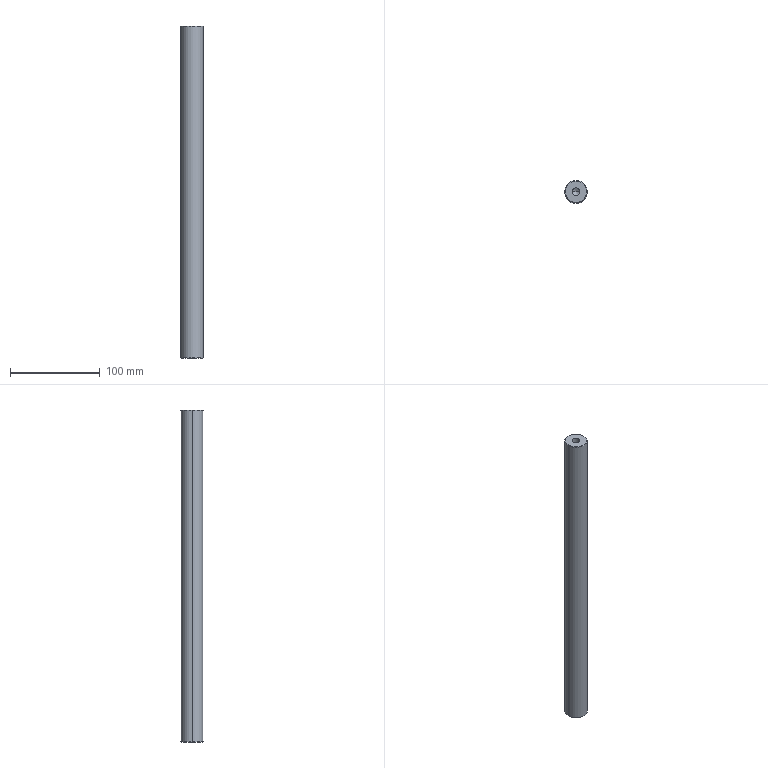Part | STEP file | 03-27 post B | 1 solid | 16 faces | box 25 x 25 x 370 mm | volume 178727 mm3 | cone 8 | cylinder 6 | plane 2 | commonest cylinder face diameters 8.5 x4 25 x2
STEP:
#1=CARTESIAN_POINT('',(4.25,0.,24.5));
#2=VERTEX_POINT('',#1);
#3=CARTESIAN_POINT('',(-4.25,0.,24.5));
#4=VERTEX_POINT('',#3);
#5=CARTESIAN_POINT('',(0.,0.,24.5));
#6=DIRECTION('',(0.,0.,-1.));
#7=DIRECTION('',(-1.,0.,0.));
#8=AXIS2_PLACEMENT_3D('',#5,#6,#7);
#9=CIRCLE('',#8,4.25);
#10=EDGE_CURVE('',#2,#4,#9,.T.);
#11=ORIENTED_EDGE('',*,*,#10,.F.);
#12=CARTESIAN_POINT('',(4.25,0.,0.));
#13=VERTEX_POINT('',#12);
#14=CARTESIAN_POINT('',(4.25,0.,0.));
#15=DIRECTION('',(0.,0.,-1.));
#16=VECTOR('',#15,1000.);
#17=LINE('',#14,#16);
#18=EDGE_CURVE('',#2,#13,#17,.T.);
#19=ORIENTED_EDGE('',*,*,#18,.T.);
#20=CARTESIAN_POINT('',(-4.25,0.,0.));
#21=VERTEX_POINT('',#20);
#22=CARTESIAN_POINT('',(0.,0.,0.));
#23=DIRECTION('',(0.,0.,-1.));
#24=DIRECTION('',(-1.,0.,0.));
#25=AXIS2_PLACEMENT_3D('',#22,#23,#24);
#26=CIRCLE('',#25,4.25);
#27=EDGE_CURVE('',#13,#21,#26,.T.);
#28=ORIENTED_EDGE('',*,*,#27,.T.);
#29=CARTESIAN_POINT('',(-4.25,0.,0.));
#30=DIRECTION('',(0.,0.,-1.));
#31=VECTOR('',#30,1000.);
#32=LINE('',#29,#31);
#33=EDGE_CURVE('',#4,#21,#32,.T.);
#34=ORIENTED_EDGE('',*,*,#33,.F.);
#35=EDGE_LOOP('',(#11,#19,#28,#34));
#36=FACE_OUTER_BOUND('',#35,.T.);
#37=CARTESIAN_POINT('',(0.,0.,0.));
#38=DIRECTION('',(0.,0.,-1.));
#39=DIRECTION('',(-1.,0.,0.));
#40=AXIS2_PLACEMENT_3D('',#37,#38,#39);
#41=CYLINDRICAL_SURFACE('',#40,4.25);
#42=ADVANCED_FACE('',(#36),#41,.F.);
#43=CARTESIAN_POINT('',(0.,0.,27.054));
#44=VERTEX_POINT('',#43);
#45=CARTESIAN_POINT('',(-4.25,0.,24.5));
#46=DIRECTION('',(-0.8572,0.,-0.515));
#47=VECTOR('',#46,1000.);
#48=LINE('',#45,#47);
#49=EDGE_CURVE('',#44,#4,#48,.T.);
#50=ORIENTED_EDGE('',*,*,#49,.F.);
#51=CARTESIAN_POINT('',(4.25,0.,24.5));
#52=DIRECTION('',(0.8572,0.,-0.515));
#53=VECTOR('',#52,1000.);
#54=LINE('',#51,#53);
#55=EDGE_CURVE('',#44,#2,#54,.T.);
#56=ORIENTED_EDGE('',*,*,#55,.T.);
#57=ORIENTED_EDGE('',*,*,#10,.T.);
#58=EDGE_LOOP('',(#50,#56,#57));
#59=FACE_OUTER_BOUND('',#58,.T.);
#60=CARTESIAN_POINT('',(0.,0.,24.5));
#61=DIRECTION('',(0.,0.,-1.));
#62=DIRECTION('',(-1.,0.,0.));
#63=AXIS2_PLACEMENT_3D('',#60,#61,#62);
#64=CONICAL_SURFACE('',#63,4.25,1.03);
#65=ADVANCED_FACE('',(#59),#64,.F.);
#66=CARTESIAN_POINT('',(-4.25,0.,345.5));
#67=VERTEX_POINT('',#66);
#68=CARTESIAN_POINT('',(4.25,0.,345.5));
#69=VERTEX_POINT('',#68);
#70=CARTESIAN_POINT('',(0.,0.,345.5));
#71=DIRECTION('',(0.,0.,1.));
#72=DIRECTION('',(1.,0.,0.));
#73=AXIS2_PLACEMENT_3D('',#70,#71,#72);
#74=CIRCLE('',#73,4.25);
#75=EDGE_CURVE('',#67,#69,#74,.T.);
#76=ORIENTED_EDGE('',*,*,#75,.F.);
#77=CARTESIAN_POINT('',(-4.25,0.,370.));
#78=VERTEX_POINT('',#77);
#79=CARTESIAN_POINT('',(-4.25,0.,370.));
#80=DIRECTION('',(0.,0.,1.));
#81=VECTOR('',#80,1000.);
#82=LINE('',#79,#81);
#83=EDGE_CURVE('',#67,#78,#82,.T.);
#84=ORIENTED_EDGE('',*,*,#83,.T.);
#85=CARTESIAN_POINT('',(4.25,0.,370.));
#86=VERTEX_POINT('',#85);
#87=CARTESIAN_POINT('',(0.,0.,370.));
#88=DIRECTION('',(0.,0.,1.));
#89=DIRECTION('',(1.,0.,0.));
#90=AXIS2_PLACEMENT_3D('',#87,#88,#89);
#91=CIRCLE('',#90,4.25);
#92=EDGE_CURVE('',#78,#86,#91,.T.);
#93=ORIENTED_EDGE('',*,*,#92,.T.);
#94=CARTESIAN_POINT('',(4.25,0.,370.));
#95=DIRECTION('',(0.,0.,1.));
#96=VECTOR('',#95,1000.);
#97=LINE('',#94,#96);
#98=EDGE_CURVE('',#69,#86,#97,.T.);
#99=ORIENTED_EDGE('',*,*,#98,.F.);
#100=EDGE_LOOP('',(#76,#84,#93,#99));
#101=FACE_OUTER_BOUND('',#100,.T.);
#102=CARTESIAN_POINT('',(0.,0.,370.));
#103=DIRECTION('',(0.,0.,1.));
#104=DIRECTION('',(1.,0.,0.));
#105=AXIS2_PLACEMENT_3D('',#102,#103,#104);
#106=CYLINDRICAL_SURFACE('',#105,4.25);
#107=ADVANCED_FACE('',(#101),#106,.F.);
#108=CARTESIAN_POINT('',(0.,0.,342.946));
#109=VERTEX_POINT('',#108);
#110=CARTESIAN_POINT('',(4.25,0.,345.5));
#111=DIRECTION('',(0.8572,0.,0.515));
#112=VECTOR('',#111,1000.);
#113=LINE('',#110,#112);
#114=EDGE_CURVE('',#109,#69,#113,.T.);
#115=ORIENTED_EDGE('',*,*,#114,.F.);
#116=CARTESIAN_POINT('',(-4.25,0.,345.5));
#117=DIRECTION('',(-0.8572,0.,0.515));
#118=VECTOR('',#117,1000.);
#119=LINE('',#116,#118);
#120=EDGE_CURVE('',#109,#67,#119,.T.);
#121=ORIENTED_EDGE('',*,*,#120,.T.);
#122=ORIENTED_EDGE('',*,*,#75,.T.);
#123=EDGE_LOOP('',(#115,#121,#122));
#124=FACE_OUTER_BOUND('',#123,.T.);
#125=CARTESIAN_POINT('',(0.,0.,345.5));
#126=DIRECTION('',(0.,0.,1.));
#127=DIRECTION('',(1.,0.,0.));
#128=AXIS2_PLACEMENT_3D('',#125,#126,#127);
#129=CONICAL_SURFACE('',#128,4.25,1.03);
#130=ADVANCED_FACE('',(#124),#129,.F.);
#131=CARTESIAN_POINT('',(12.,0.,370.));
#132=VERTEX_POINT('',#131);
#133=CARTESIAN_POINT('',(-12.,0.,370.));
#134=VERTEX_POINT('',#133);
#135=CARTESIAN_POINT('',(0.,0.,370.));
#136=DIRECTION('',(0.,0.,1.));
#137=DIRECTION('',(1.,0.,0.));
#138=AXIS2_PLACEMENT_3D('',#135,#136,#137);
#139=CIRCLE('',#138,12.);
#140=EDGE_CURVE('',#132,#134,#139,.T.);
#141=ORIENTED_EDGE('',*,*,#140,.F.);
#142=CARTESIAN_POINT('',(12.5,0.,369.5));
#143=VERTEX_POINT('',#142);
#144=CARTESIAN_POINT('',(12.,0.,370.));
#145=DIRECTION('',(0.7071,0.,-0.7071));
#146=VECTOR('',#145,1000.);
#147=LINE('',#144,#146);
#148=EDGE_CURVE('',#132,#143,#147,.T.);
#149=ORIENTED_EDGE('',*,*,#148,.T.);
#150=CARTESIAN_POINT('',(-12.5,0.,369.5));
#151=VERTEX_POINT('',#150);
#152=CARTESIAN_POINT('',(0.,0.,369.5));
#153=DIRECTION('',(0.,0.,-1.));
#154=DIRECTION('',(1.,0.,0.));
#155=AXIS2_PLACEMENT_3D('',#152,#153,#154);
#156=CIRCLE('',#155,12.5);
#157=EDGE_CURVE('',#151,#143,#156,.T.);
#158=ORIENTED_EDGE('',*,*,#157,.F.);
#159=CARTESIAN_POINT('',(-12.,0.,370.));
#160=DIRECTION('',(-0.7071,0.,-0.7071));
#161=VECTOR('',#160,1000.);
#162=LINE('',#159,#161);
#163=EDGE_CURVE('',#134,#151,#162,.T.);
#164=ORIENTED_EDGE('',*,*,#163,.F.);
#165=EDGE_LOOP('',(#141,#149,#158,#164));
#166=FACE_OUTER_BOUND('',#165,.T.);
#167=CARTESIAN_POINT('',(0.,0.,370.));
#168=DIRECTION('',(0.,0.,-1.));
#169=DIRECTION('',(-1.,0.,0.));
#170=AXIS2_PLACEMENT_3D('',#167,#168,#169);
#171=CONICAL_SURFACE('',#170,12.,0.7854);
#172=ADVANCED_FACE('',(#166),#171,.T.);
#173=CARTESIAN_POINT('',(-12.,0.,0.));
#174=VERTEX_POINT('',#173);
#175=CARTESIAN_POINT('',(12.,0.,0.));
#176=VERTEX_POINT('',#175);
#177=CARTESIAN_POINT('',(0.,0.,0.));
#178=DIRECTION('',(0.,0.,-1.));
#179=DIRECTION('',(1.,0.,0.));
#180=AXIS2_PLACEMENT_3D('',#177,#178,#179);
#181=CIRCLE('',#180,12.);
#182=EDGE_CURVE('',#174,#176,#181,.T.);
#183=ORIENTED_EDGE('',*,*,#182,.F.);
#184=CARTESIAN_POINT('',(-12.5,0.,0.5));
#185=VERTEX_POINT('',#184);
#186=CARTESIAN_POINT('',(-12.5,0.,0.5));
#187=DIRECTION('',(-0.7071,0.,0.7071));
#188=VECTOR('',#187,1000.);
#189=LINE('',#186,#188);
#190=EDGE_CURVE('',#174,#185,#189,.T.);
#191=ORIENTED_EDGE('',*,*,#190,.T.);
#192=CARTESIAN_POINT('',(12.5,0.,0.5));
#193=VERTEX_POINT('',#192);
#194=CARTESIAN_POINT('',(0.,0.,0.5));
#195=DIRECTION('',(0.,0.,1.));
#196=DIRECTION('',(1.,0.,0.));
#197=AXIS2_PLACEMENT_3D('',#194,#195,#196);
#198=CIRCLE('',#197,12.5);
#199=EDGE_CURVE('',#193,#185,#198,.T.);
#200=ORIENTED_EDGE('',*,*,#199,.F.);
#201=CARTESIAN_POINT('',(12.5,0.,0.5));
#202=DIRECTION('',(0.7071,0.,0.7071));
#203=VECTOR('',#202,1000.);
#204=LINE('',#201,#203);
#205=EDGE_CURVE('',#176,#193,#204,.T.);
#206=ORIENTED_EDGE('',*,*,#205,.F.);
#207=EDGE_LOOP('',(#183,#191,#200,#206));
#208=FACE_OUTER_BOUND('',#207,.T.);
#209=CARTESIAN_POINT('',(0.,0.,0.5));
#210=DIRECTION('',(0.,0.,1.));
#211=DIRECTION('',(1.,0.,0.));
#212=AXIS2_PLACEMENT_3D('',#209,#210,#211);
#213=CONICAL_SURFACE('',#212,12.5,0.7854);
#214=ADVANCED_FACE('',(#208),#213,.T.);
#215=ORIENTED_EDGE('',*,*,#157,.T.);
#216=CARTESIAN_POINT('',(12.5,0.,370.));
#217=DIRECTION('',(0.,0.,-1.));
#218=VECTOR('',#217,1000.);
#219=LINE('',#216,#218);
#220=EDGE_CURVE('',#143,#193,#219,.T.);
#221=ORIENTED_EDGE('',*,*,#220,.T.);
#222=ORIENTED_EDGE('',*,*,#199,.T.);
#223=CARTESIAN_POINT('',(-12.5,0.,370.));
#224=DIRECTION('',(0.,0.,-1.));
#225=VECTOR('',#224,1000.);
#226=LINE('',#223,#225);
#227=EDGE_CURVE('',#151,#185,#226,.T.);
#228=ORIENTED_EDGE('',*,*,#227,.F.);
#229=EDGE_LOOP('',(#215,#221,#222,#228));
#230=FACE_OUTER_BOUND('',#229,.T.);
#231=CARTESIAN_POINT('',(0.,0.,370.));
#232=DIRECTION('',(0.,0.,-1.));
#233=DIRECTION('',(-1.,0.,0.));
#234=AXIS2_PLACEMENT_3D('',#231,#232,#233);
#235=CYLINDRICAL_SURFACE('',#234,12.5);
#236=ADVANCED_FACE('',(#230),#235,.T.);
#237=ORIENTED_EDGE('',*,*,#220,.F.);
#238=CARTESIAN_POINT('',(0.,0.,369.5));
#239=DIRECTION('',(0.,0.,-1.));
#240=DIRECTION('',(1.,0.,0.));
#241=AXIS2_PLACEMENT_3D('',#238,#239,#240);
#242=CIRCLE('',#241,12.5);
#243=EDGE_CURVE('',#143,#151,#242,.T.);
#244=ORIENTED_EDGE('',*,*,#243,.T.);
#245=ORIENTED_EDGE('',*,*,#227,.T.);
#246=CARTESIAN_POINT('',(0.,0.,0.5));
#247=DIRECTION('',(0.,0.,1.));
#248=DIRECTION('',(1.,0.,0.));
#249=AXIS2_PLACEMENT_3D('',#246,#247,#248);
#250=CIRCLE('',#249,12.5);
#251=EDGE_CURVE('',#185,#193,#250,.T.);
#252=ORIENTED_EDGE('',*,*,#251,.T.);
#253=EDGE_LOOP('',(#237,#244,#245,#252));
#254=FACE_OUTER_BOUND('',#253,.T.);
#255=CARTESIAN_POINT('',(0.,0.,370.));
#256=DIRECTION('',(0.,0.,-1.));
#257=DIRECTION('',(-1.,0.,0.));
#258=AXIS2_PLACEMENT_3D('',#255,#256,#257);
#259=CYLINDRICAL_SURFACE('',#258,12.5);
#260=ADVANCED_FACE('',(#254),#259,.T.);
#261=CARTESIAN_POINT('',(0.,0.,370.));
#262=DIRECTION('',(0.,0.,1.));
#263=DIRECTION('',(1.,0.,0.));
#264=AXIS2_PLACEMENT_3D('',#261,#262,#263);
#265=CIRCLE('',#264,4.25);
#266=EDGE_CURVE('',#86,#78,#265,.T.);
#267=ORIENTED_EDGE('',*,*,#266,.F.);
#268=ORIENTED_EDGE('',*,*,#92,.F.);
#269=EDGE_LOOP('',(#267,#268));
#270=FACE_BOUND('',#269,.T.);
#271=CARTESIAN_POINT('',(0.,0.,370.));
#272=DIRECTION('',(0.,0.,1.));
#273=DIRECTION('',(1.,0.,0.));
#274=AXIS2_PLACEMENT_3D('',#271,#272,#273);
#275=CIRCLE('',#274,12.);
#276=EDGE_CURVE('',#134,#132,#275,.T.);
#277=ORIENTED_EDGE('',*,*,#276,.T.);
#278=ORIENTED_EDGE('',*,*,#140,.T.);
#279=EDGE_LOOP('',(#277,#278));
#280=FACE_OUTER_BOUND('',#279,.T.);
#281=CARTESIAN_POINT('',(0.,0.,370.));
#282=DIRECTION('',(0.,0.,1.));
#283=DIRECTION('',(1.,0.,0.));
#284=AXIS2_PLACEMENT_3D('',#281,#282,#283);
#285=PLANE('',#284);
#286=ADVANCED_FACE('',(#270,#280),#285,.T.);
#287=CARTESIAN_POINT('',(0.,0.,0.));
#288=DIRECTION('',(0.,0.,-1.));
#289=DIRECTION('',(-1.,0.,0.));
#290=AXIS2_PLACEMENT_3D('',#287,#288,#289);
#291=CIRCLE('',#290,4.25);
#292=EDGE_CURVE('',#21,#13,#291,.T.);
#293=ORIENTED_EDGE('',*,*,#292,.F.);
#294=ORIENTED_EDGE('',*,*,#27,.F.);
#295=EDGE_LOOP('',(#293,#294));
#296=FACE_BOUND('',#295,.T.);
#297=CARTESIAN_POINT('',(0.,0.,0.));
#298=DIRECTION('',(0.,0.,-1.));
#299=DIRECTION('',(1.,0.,0.));
#300=AXIS2_PLACEMENT_3D('',#297,#298,#299);
#301=CIRCLE('',#300,12.);
#302=EDGE_CURVE('',#176,#174,#301,.T.);
#303=ORIENTED_EDGE('',*,*,#302,.T.);
#304=ORIENTED_EDGE('',*,*,#182,.T.);
#305=EDGE_LOOP('',(#303,#304));
#306=FACE_OUTER_BOUND('',#305,.T.);
#307=CARTESIAN_POINT('',(0.,0.,0.));
#308=DIRECTION('',(0.,0.,1.));
#309=DIRECTION('',(1.,0.,0.));
#310=AXIS2_PLACEMENT_3D('',#307,#308,#309);
#311=PLANE('',#310);
#312=ADVANCED_FACE('',(#296,#306),#311,.F.);
#313=ORIENTED_EDGE('',*,*,#190,.F.);
#314=ORIENTED_EDGE('',*,*,#302,.F.);
#315=ORIENTED_EDGE('',*,*,#205,.T.);
#316=ORIENTED_EDGE('',*,*,#251,.F.);
#317=EDGE_LOOP('',(#313,#314,#315,#316));
#318=FACE_OUTER_BOUND('',#317,.T.);
#319=CARTESIAN_POINT('',(0.,0.,0.5));
#320=DIRECTION('',(0.,0.,1.));
#321=DIRECTION('',(1.,0.,0.));
#322=AXIS2_PLACEMENT_3D('',#319,#320,#321);
#323=CONICAL_SURFACE('',#322,12.5,0.7854);
#324=ADVANCED_FACE('',(#318),#323,.T.);
#325=ORIENTED_EDGE('',*,*,#148,.F.);
#326=ORIENTED_EDGE('',*,*,#276,.F.);
#327=ORIENTED_EDGE('',*,*,#163,.T.);
#328=ORIENTED_EDGE('',*,*,#243,.F.);
#329=EDGE_LOOP('',(#325,#326,#327,#328));
#330=FACE_OUTER_BOUND('',#329,.T.);
#331=CARTESIAN_POINT('',(0.,0.,370.));
#332=DIRECTION('',(0.,0.,-1.));
#333=DIRECTION('',(-1.,0.,0.));
#334=AXIS2_PLACEMENT_3D('',#331,#332,#333);
#335=CONICAL_SURFACE('',#334,12.,0.7854);
#336=ADVANCED_FACE('',(#330),#335,.T.);
#337=ORIENTED_EDGE('',*,*,#120,.F.);
#338=ORIENTED_EDGE('',*,*,#114,.T.);
#339=CARTESIAN_POINT('',(0.,0.,345.5));
#340=DIRECTION('',(0.,0.,1.));
#341=DIRECTION('',(1.,0.,0.));
#342=AXIS2_PLACEMENT_3D('',#339,#340,#341);
#343=CIRCLE('',#342,4.25);
#344=EDGE_CURVE('',#69,#67,#343,.T.);
#345=ORIENTED_EDGE('',*,*,#344,.T.);
#346=EDGE_LOOP('',(#337,#338,#345));
#347=FACE_OUTER_BOUND('',#346,.T.);
#348=CARTESIAN_POINT('',(0.,0.,345.5));
#349=DIRECTION('',(0.,0.,1.));
#350=DIRECTION('',(1.,0.,0.));
#351=AXIS2_PLACEMENT_3D('',#348,#349,#350);
#352=CONICAL_SURFACE('',#351,4.25,1.03);
#353=ADVANCED_FACE('',(#347),#352,.F.);
#354=ORIENTED_EDGE('',*,*,#83,.F.);
#355=ORIENTED_EDGE('',*,*,#344,.F.);
#356=ORIENTED_EDGE('',*,*,#98,.T.);
#357=ORIENTED_EDGE('',*,*,#266,.T.);
#358=EDGE_LOOP('',(#354,#355,#356,#357));
#359=FACE_OUTER_BOUND('',#358,.T.);
#360=CARTESIAN_POINT('',(0.,0.,370.));
#361=DIRECTION('',(0.,0.,1.));
#362=DIRECTION('',(1.,0.,0.));
#363=AXIS2_PLACEMENT_3D('',#360,#361,#362);
#364=CYLINDRICAL_SURFACE('',#363,4.25);
#365=ADVANCED_FACE('',(#359),#364,.F.);
#366=ORIENTED_EDGE('',*,*,#55,.F.);
#367=ORIENTED_EDGE('',*,*,#49,.T.);
#368=CARTESIAN_POINT('',(0.,0.,24.5));
#369=DIRECTION('',(0.,0.,-1.));
#370=DIRECTION('',(-1.,0.,0.));
#371=AXIS2_PLACEMENT_3D('',#368,#369,#370);
#372=CIRCLE('',#371,4.25);
#373=EDGE_CURVE('',#4,#2,#372,.T.);
#374=ORIENTED_EDGE('',*,*,#373,.T.);
#375=EDGE_LOOP('',(#366,#367,#374));
#376=FACE_OUTER_BOUND('',#375,.T.);
#377=CARTESIAN_POINT('',(0.,0.,24.5));
#378=DIRECTION('',(0.,0.,-1.));
#379=DIRECTION('',(-1.,0.,0.));
#380=AXIS2_PLACEMENT_3D('',#377,#378,#379);
#381=CONICAL_SURFACE('',#380,4.25,1.03);
#382=ADVANCED_FACE('',(#376),#381,.F.);
#383=ORIENTED_EDGE('',*,*,#18,.F.);
#384=ORIENTED_EDGE('',*,*,#373,.F.);
#385=ORIENTED_EDGE('',*,*,#33,.T.);
#386=ORIENTED_EDGE('',*,*,#292,.T.);
#387=EDGE_LOOP('',(#383,#384,#385,#386));
#388=FACE_OUTER_BOUND('',#387,.T.);
#389=CARTESIAN_POINT('',(0.,0.,0.));
#390=DIRECTION('',(0.,0.,-1.));
#391=DIRECTION('',(-1.,0.,0.));
#392=AXIS2_PLACEMENT_3D('',#389,#390,#391);
#393=CYLINDRICAL_SURFACE('',#392,4.25);
#394=ADVANCED_FACE('',(#388),#393,.F.);
#395=CLOSED_SHELL('',(#42,#65,#107,#130,#172,#214,#236,#260,#286,#312,#324,#336,#353,#365,#382,#394));
#396=MANIFOLD_SOLID_BREP('',#395);
#397=CARTESIAN_POINT('',(0.,0.,0.));
#398=DIRECTION('',(0.,0.,1.));
#399=DIRECTION('',(1.,0.,0.));
#400=AXIS2_PLACEMENT_3D('',#397,#398,#399);
#401=(LENGTH_UNIT()NAMED_UNIT(*)SI_UNIT(.MILLI.,.METRE.));
#402=UNCERTAINTY_MEASURE_WITH_UNIT(LENGTH_MEASURE(0.00001),#401,'','');
#403=(NAMED_UNIT(*)PLANE_ANGLE_UNIT()SI_UNIT($,.RADIAN.));
#404=(NAMED_UNIT(*)SI_UNIT($,.STERADIAN.)SOLID_ANGLE_UNIT());
#405=(GEOMETRIC_REPRESENTATION_CONTEXT(3)GLOBAL_UNCERTAINTY_ASSIGNED_CONTEXT((#402))GLOBAL_UNIT_ASSIGNED_CONTEXT((#401,#403,#404))REPRESENTATION_CONTEXT('',''));
#406=ADVANCED_BREP_SHAPE_REPRESENTATION('',(#396,#400),#405);